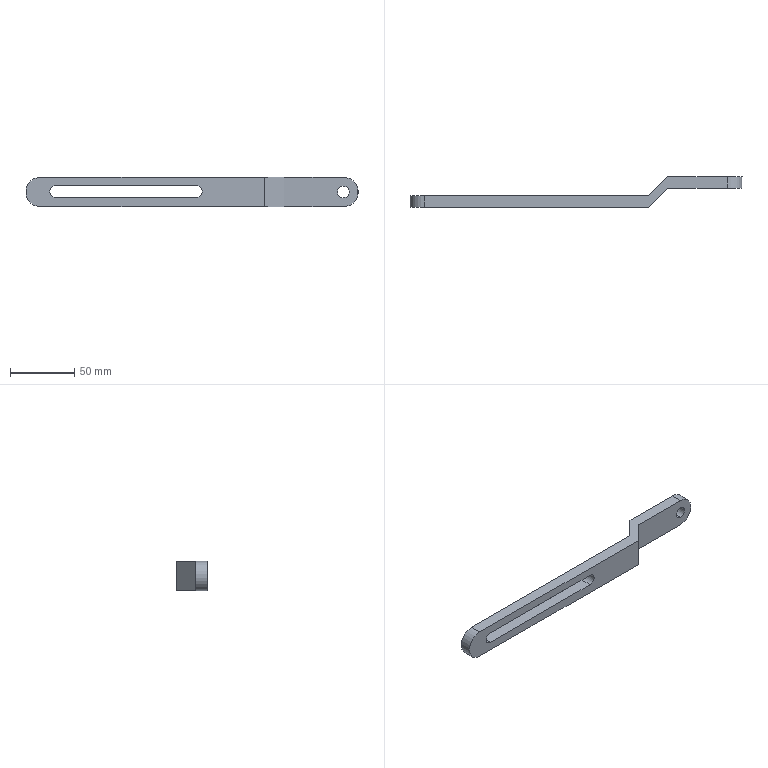Part | SolidWorks | features BaseBody 1 | 1 solid | 17 faces | box 258.849 x 23.849 x 23 mm | volume 42505 mm3 | plane 10 | cylinder 7 | commonest cylinder face diameters 9 x5 23 x2
STEP:
#1=CARTESIAN_POINT('',(247.349,14.849,7.));
#2=VERTEX_POINT('',#1);
#3=CARTESIAN_POINT('',(247.349,14.849,16.));
#4=VERTEX_POINT('',#3);
#5=CARTESIAN_POINT('',(247.349,14.849,11.5));
#6=DIRECTION('',(0.,-1.,0.));
#7=DIRECTION('',(0.,0.,-1.));
#8=AXIS2_PLACEMENT_3D('',#5,#6,#7);
#9=CIRCLE('',#8,4.5);
#10=EDGE_CURVE('',#2,#4,#9,.T.);
#11=ORIENTED_EDGE('',*,*,#10,.F.);
#12=CARTESIAN_POINT('',(247.349,5.849,7.));
#13=VERTEX_POINT('',#12);
#14=CARTESIAN_POINT('',(247.349,14.849,7.));
#15=DIRECTION('',(0.,-1.,0.));
#16=VECTOR('',#15,1000.);
#17=LINE('',#14,#16);
#18=EDGE_CURVE('',#2,#13,#17,.T.);
#19=ORIENTED_EDGE('',*,*,#18,.T.);
#20=CARTESIAN_POINT('',(247.349,5.849,16.));
#21=VERTEX_POINT('',#20);
#22=CARTESIAN_POINT('',(247.349,5.849,11.5));
#23=DIRECTION('',(0.,1.,0.));
#24=DIRECTION('',(-1.,0.,0.));
#25=AXIS2_PLACEMENT_3D('',#22,#23,#24);
#26=CIRCLE('',#25,4.5);
#27=EDGE_CURVE('',#21,#13,#26,.T.);
#28=ORIENTED_EDGE('',*,*,#27,.F.);
#29=CARTESIAN_POINT('',(247.349,14.849,16.));
#30=DIRECTION('',(0.,-1.,0.));
#31=VECTOR('',#30,1000.);
#32=LINE('',#29,#31);
#33=EDGE_CURVE('',#4,#21,#32,.T.);
#34=ORIENTED_EDGE('',*,*,#33,.F.);
#35=EDGE_LOOP('',(#11,#19,#28,#34));
#36=FACE_OUTER_BOUND('',#35,.T.);
#37=CARTESIAN_POINT('',(247.349,14.849,11.5));
#38=DIRECTION('',(0.,-1.,0.));
#39=DIRECTION('',(0.,0.,1.));
#40=AXIS2_PLACEMENT_3D('',#37,#38,#39);
#41=CYLINDRICAL_SURFACE('',#40,4.5);
#42=ADVANCED_FACE('',(#36),#41,.F.);
#43=CARTESIAN_POINT('',(22.998,-9.,16.35));
#44=VERTEX_POINT('',#43);
#45=CARTESIAN_POINT('',(23.,-9.,7.35));
#46=VERTEX_POINT('',#45);
#47=CARTESIAN_POINT('',(23.,-9.,11.85));
#48=DIRECTION('',(0.,-1.,0.));
#49=DIRECTION('',(-1.,0.,0.));
#50=AXIS2_PLACEMENT_3D('',#47,#48,#49);
#51=CIRCLE('',#50,4.5);
#52=EDGE_CURVE('',#44,#46,#51,.T.);
#53=ORIENTED_EDGE('',*,*,#52,.T.);
#54=CARTESIAN_POINT('',(23.,0.,7.35));
#55=VERTEX_POINT('',#54);
#56=CARTESIAN_POINT('',(23.,-23.,7.35));
#57=DIRECTION('',(0.,1.,0.));
#58=VECTOR('',#57,1000.);
#59=LINE('',#56,#58);
#60=EDGE_CURVE('',#46,#55,#59,.T.);
#61=ORIENTED_EDGE('',*,*,#60,.T.);
#62=CARTESIAN_POINT('',(22.998,0.,16.35));
#63=VERTEX_POINT('',#62);
#64=CARTESIAN_POINT('',(23.,0.,11.85));
#65=DIRECTION('',(0.,-1.,0.));
#66=DIRECTION('',(-1.,0.,0.));
#67=AXIS2_PLACEMENT_3D('',#64,#65,#66);
#68=CIRCLE('',#67,4.5);
#69=EDGE_CURVE('',#63,#55,#68,.T.);
#70=ORIENTED_EDGE('',*,*,#69,.F.);
#71=CARTESIAN_POINT('',(22.998,-23.,16.35));
#72=DIRECTION('',(0.,-1.,0.));
#73=VECTOR('',#72,1000.);
#74=LINE('',#71,#73);
#75=EDGE_CURVE('',#63,#44,#74,.T.);
#76=ORIENTED_EDGE('',*,*,#75,.T.);
#77=EDGE_LOOP('',(#53,#61,#70,#76));
#78=FACE_OUTER_BOUND('',#77,.T.);
#79=CARTESIAN_POINT('',(23.,-23.,11.85));
#80=DIRECTION('',(0.,1.,0.));
#81=DIRECTION('',(0.,0.,-1.));
#82=AXIS2_PLACEMENT_3D('',#79,#80,#81);
#83=CYLINDRICAL_SURFACE('',#82,4.5);
#84=ADVANCED_FACE('',(#78),#83,.F.);
#85=CARTESIAN_POINT('',(133.002,-9.,7.407));
#86=VERTEX_POINT('',#85);
#87=CARTESIAN_POINT('',(132.998,-9.,16.407));
#88=VERTEX_POINT('',#87);
#89=CARTESIAN_POINT('',(133.,-9.,11.907));
#90=DIRECTION('',(0.,-1.,0.));
#91=DIRECTION('',(-1.,0.,0.));
#92=AXIS2_PLACEMENT_3D('',#89,#90,#91);
#93=CIRCLE('',#92,4.5);
#94=EDGE_CURVE('',#86,#88,#93,.T.);
#95=ORIENTED_EDGE('',*,*,#94,.T.);
#96=CARTESIAN_POINT('',(132.998,0.,16.407));
#97=VERTEX_POINT('',#96);
#98=CARTESIAN_POINT('',(132.998,-23.,16.407));
#99=DIRECTION('',(0.,-1.,0.));
#100=VECTOR('',#99,1000.);
#101=LINE('',#98,#100);
#102=EDGE_CURVE('',#97,#88,#101,.T.);
#103=ORIENTED_EDGE('',*,*,#102,.F.);
#104=CARTESIAN_POINT('',(133.002,0.,7.407));
#105=VERTEX_POINT('',#104);
#106=CARTESIAN_POINT('',(133.,0.,11.907));
#107=DIRECTION('',(0.,-1.,0.));
#108=DIRECTION('',(-1.,0.,0.));
#109=AXIS2_PLACEMENT_3D('',#106,#107,#108);
#110=CIRCLE('',#109,4.5);
#111=EDGE_CURVE('',#105,#97,#110,.T.);
#112=ORIENTED_EDGE('',*,*,#111,.F.);
#113=CARTESIAN_POINT('',(133.002,-23.,7.407));
#114=DIRECTION('',(0.,-1.,0.));
#115=VECTOR('',#114,1000.);
#116=LINE('',#113,#115);
#117=EDGE_CURVE('',#105,#86,#116,.T.);
#118=ORIENTED_EDGE('',*,*,#117,.T.);
#119=EDGE_LOOP('',(#95,#103,#112,#118));
#120=FACE_OUTER_BOUND('',#119,.T.);
#121=CARTESIAN_POINT('',(133.,-23.,11.907));
#122=DIRECTION('',(0.,1.,0.));
#123=DIRECTION('',(0.,0.,-1.));
#124=AXIS2_PLACEMENT_3D('',#121,#122,#123);
#125=CYLINDRICAL_SURFACE('',#124,4.5);
#126=ADVANCED_FACE('',(#120),#125,.F.);
#127=CARTESIAN_POINT('',(23.002,-9.,7.35));
#128=VERTEX_POINT('',#127);
#129=CARTESIAN_POINT('',(0.008065,-9.,7.338));
#130=DIRECTION('',(1.,0.,0.000515));
#131=VECTOR('',#130,1000.);
#132=LINE('',#129,#131);
#133=EDGE_CURVE('',#128,#86,#132,.T.);
#134=ORIENTED_EDGE('',*,*,#133,.T.);
#135=ORIENTED_EDGE('',*,*,#117,.F.);
#136=CARTESIAN_POINT('',(23.002,0.,7.35));
#137=VERTEX_POINT('',#136);
#138=CARTESIAN_POINT('',(23.002,0.,7.35));
#139=DIRECTION('',(1.,0.,0.000515));
#140=VECTOR('',#139,1000.);
#141=LINE('',#138,#140);
#142=EDGE_CURVE('',#137,#105,#141,.T.);
#143=ORIENTED_EDGE('',*,*,#142,.F.);
#144=CARTESIAN_POINT('',(23.002,-23.,7.35));
#145=DIRECTION('',(0.,-1.,0.));
#146=VECTOR('',#145,1000.);
#147=LINE('',#144,#146);
#148=EDGE_CURVE('',#137,#128,#147,.T.);
#149=ORIENTED_EDGE('',*,*,#148,.T.);
#150=EDGE_LOOP('',(#134,#135,#143,#149));
#151=FACE_OUTER_BOUND('',#150,.T.);
#152=CARTESIAN_POINT('',(23.002,-23.,7.35));
#153=DIRECTION('',(-0.000515,0.,1.));
#154=DIRECTION('',(0.,1.,0.));
#155=AXIS2_PLACEMENT_3D('',#152,#153,#154);
#156=PLANE('',#155);
#157=ADVANCED_FACE('',(#151),#156,.T.);
#158=ORIENTED_EDGE('',*,*,#60,.F.);
#159=CARTESIAN_POINT('',(23.,-9.,11.85));
#160=DIRECTION('',(0.,-1.,0.));
#161=DIRECTION('',(-1.,0.,0.));
#162=AXIS2_PLACEMENT_3D('',#159,#160,#161);
#163=CIRCLE('',#162,4.5);
#164=EDGE_CURVE('',#46,#128,#163,.T.);
#165=ORIENTED_EDGE('',*,*,#164,.T.);
#166=ORIENTED_EDGE('',*,*,#148,.F.);
#167=CARTESIAN_POINT('',(23.,0.,11.85));
#168=DIRECTION('',(0.,-1.,0.));
#169=DIRECTION('',(-1.,0.,0.));
#170=AXIS2_PLACEMENT_3D('',#167,#168,#169);
#171=CIRCLE('',#170,4.5);
#172=EDGE_CURVE('',#55,#137,#171,.T.);
#173=ORIENTED_EDGE('',*,*,#172,.F.);
#174=EDGE_LOOP('',(#158,#165,#166,#173));
#175=FACE_OUTER_BOUND('',#174,.T.);
#176=CARTESIAN_POINT('',(23.,-23.,11.85));
#177=DIRECTION('',(0.,1.,0.));
#178=DIRECTION('',(0.,0.,-1.));
#179=AXIS2_PLACEMENT_3D('',#176,#177,#178);
#180=CYLINDRICAL_SURFACE('',#179,4.5);
#181=ADVANCED_FACE('',(#175),#180,.F.);
#182=CARTESIAN_POINT('',(0.003431,-9.,16.338));
#183=DIRECTION('',(-1.,0.,-0.000515));
#184=VECTOR('',#183,1000.);
#185=LINE('',#182,#184);
#186=EDGE_CURVE('',#88,#44,#185,.T.);
#187=ORIENTED_EDGE('',*,*,#186,.T.);
#188=ORIENTED_EDGE('',*,*,#75,.F.);
#189=CARTESIAN_POINT('',(132.998,0.,16.407));
#190=DIRECTION('',(-1.,0.,-0.000515));
#191=VECTOR('',#190,1000.);
#192=LINE('',#189,#191);
#193=EDGE_CURVE('',#97,#63,#192,.T.);
#194=ORIENTED_EDGE('',*,*,#193,.F.);
#195=ORIENTED_EDGE('',*,*,#102,.T.);
#196=EDGE_LOOP('',(#187,#188,#194,#195));
#197=FACE_OUTER_BOUND('',#196,.T.);
#198=CARTESIAN_POINT('',(132.998,-23.,16.407));
#199=DIRECTION('',(0.000515,0.,-1.));
#200=DIRECTION('',(0.,-1.,0.));
#201=AXIS2_PLACEMENT_3D('',#198,#199,#200);
#202=PLANE('',#201);
#203=ADVANCED_FACE('',(#197),#202,.T.);
#204=ORIENTED_EDGE('',*,*,#18,.F.);
#205=CARTESIAN_POINT('',(247.349,14.849,11.5));
#206=DIRECTION('',(0.,-1.,0.));
#207=DIRECTION('',(0.,0.,-1.));
#208=AXIS2_PLACEMENT_3D('',#205,#206,#207);
#209=CIRCLE('',#208,4.5);
#210=EDGE_CURVE('',#4,#2,#209,.T.);
#211=ORIENTED_EDGE('',*,*,#210,.F.);
#212=ORIENTED_EDGE('',*,*,#33,.T.);
#213=CARTESIAN_POINT('',(247.349,5.849,11.5));
#214=DIRECTION('',(0.,1.,0.));
#215=DIRECTION('',(-1.,0.,0.));
#216=AXIS2_PLACEMENT_3D('',#213,#214,#215);
#217=CIRCLE('',#216,4.5);
#218=EDGE_CURVE('',#13,#21,#217,.T.);
#219=ORIENTED_EDGE('',*,*,#218,.F.);
#220=EDGE_LOOP('',(#204,#211,#212,#219));
#221=FACE_OUTER_BOUND('',#220,.T.);
#222=CARTESIAN_POINT('',(247.349,14.849,11.5));
#223=DIRECTION('',(0.,-1.,0.));
#224=DIRECTION('',(0.,0.,1.));
#225=AXIS2_PLACEMENT_3D('',#222,#223,#224);
#226=CYLINDRICAL_SURFACE('',#225,4.5);
#227=ADVANCED_FACE('',(#221),#226,.F.);
#228=CARTESIAN_POINT('',(11.5,0.,0.));
#229=VERTEX_POINT('',#228);
#230=CARTESIAN_POINT('',(11.5,0.,23.));
#231=VERTEX_POINT('',#230);
#232=CARTESIAN_POINT('',(11.5,0.,11.5));
#233=DIRECTION('',(0.,1.,0.));
#234=DIRECTION('',(0.,0.,-1.));
#235=AXIS2_PLACEMENT_3D('',#232,#233,#234);
#236=CIRCLE('',#235,11.5);
#237=EDGE_CURVE('',#229,#231,#236,.T.);
#238=ORIENTED_EDGE('',*,*,#237,.F.);
#239=CARTESIAN_POINT('',(11.5,-9.,0.));
#240=VERTEX_POINT('',#239);
#241=CARTESIAN_POINT('',(11.5,0.,0.));
#242=DIRECTION('',(0.,1.,0.));
#243=VECTOR('',#242,1000.);
#244=LINE('',#241,#243);
#245=EDGE_CURVE('',#240,#229,#244,.T.);
#246=ORIENTED_EDGE('',*,*,#245,.F.);
#247=CARTESIAN_POINT('',(11.5,-9.,23.));
#248=VERTEX_POINT('',#247);
#249=CARTESIAN_POINT('',(11.5,-9.,11.5));
#250=DIRECTION('',(0.,-1.,0.));
#251=DIRECTION('',(-1.,0.,0.));
#252=AXIS2_PLACEMENT_3D('',#249,#250,#251);
#253=CIRCLE('',#252,11.5);
#254=EDGE_CURVE('',#248,#240,#253,.T.);
#255=ORIENTED_EDGE('',*,*,#254,.F.);
#256=CARTESIAN_POINT('',(11.5,-9.,23.));
#257=DIRECTION('',(0.,-1.,0.));
#258=VECTOR('',#257,1000.);
#259=LINE('',#256,#258);
#260=EDGE_CURVE('',#231,#248,#259,.T.);
#261=ORIENTED_EDGE('',*,*,#260,.F.);
#262=EDGE_LOOP('',(#238,#246,#255,#261));
#263=FACE_OUTER_BOUND('',#262,.T.);
#264=CARTESIAN_POINT('',(11.5,0.,11.5));
#265=DIRECTION('',(0.,1.,0.));
#266=DIRECTION('',(1.,0.,0.));
#267=AXIS2_PLACEMENT_3D('',#264,#265,#266);
#268=CYLINDRICAL_SURFACE('',#267,11.5);
#269=ADVANCED_FACE('',(#263),#268,.T.);
#270=CARTESIAN_POINT('',(247.349,5.849,0.));
#271=VERTEX_POINT('',#270);
#272=CARTESIAN_POINT('',(247.349,5.849,23.));
#273=VERTEX_POINT('',#272);
#274=CARTESIAN_POINT('',(247.349,5.849,11.5));
#275=DIRECTION('',(0.,-1.,0.));
#276=DIRECTION('',(-1.,0.,0.));
#277=AXIS2_PLACEMENT_3D('',#274,#275,#276);
#278=CIRCLE('',#277,11.5);
#279=EDGE_CURVE('',#271,#273,#278,.T.);
#280=ORIENTED_EDGE('',*,*,#279,.F.);
#281=CARTESIAN_POINT('',(247.349,14.849,0.));
#282=VERTEX_POINT('',#281);
#283=CARTESIAN_POINT('',(247.349,0.,0.));
#284=DIRECTION('',(0.,-1.,0.));
#285=VECTOR('',#284,1000.);
#286=LINE('',#283,#285);
#287=EDGE_CURVE('',#282,#271,#286,.T.);
#288=ORIENTED_EDGE('',*,*,#287,.F.);
#289=CARTESIAN_POINT('',(247.349,14.849,23.));
#290=VERTEX_POINT('',#289);
#291=CARTESIAN_POINT('',(247.349,14.849,11.5));
#292=DIRECTION('',(0.,1.,0.));
#293=DIRECTION('',(0.,0.,-1.));
#294=AXIS2_PLACEMENT_3D('',#291,#292,#293);
#295=CIRCLE('',#294,11.5);
#296=EDGE_CURVE('',#290,#282,#295,.T.);
#297=ORIENTED_EDGE('',*,*,#296,.F.);
#298=CARTESIAN_POINT('',(247.349,14.849,23.));
#299=DIRECTION('',(0.,1.,0.));
#300=VECTOR('',#299,1000.);
#301=LINE('',#298,#300);
#302=EDGE_CURVE('',#273,#290,#301,.T.);
#303=ORIENTED_EDGE('',*,*,#302,.F.);
#304=EDGE_LOOP('',(#280,#288,#297,#303));
#305=FACE_OUTER_BOUND('',#304,.T.);
#306=CARTESIAN_POINT('',(247.349,0.,11.5));
#307=DIRECTION('',(0.,-1.,0.));
#308=DIRECTION('',(-1.,0.,0.));
#309=AXIS2_PLACEMENT_3D('',#306,#307,#308);
#310=CYLINDRICAL_SURFACE('',#309,11.5);
#311=ADVANCED_FACE('',(#305),#310,.T.);
#312=CARTESIAN_POINT('',(186.,-9.,0.));
#313=VERTEX_POINT('',#312);
#314=CARTESIAN_POINT('',(0.,-9.,0.));
#315=DIRECTION('',(1.,0.,0.));
#316=VECTOR('',#315,1000.);
#317=LINE('',#314,#316);
#318=EDGE_CURVE('',#240,#313,#317,.T.);
#319=ORIENTED_EDGE('',*,*,#318,.F.);
#320=ORIENTED_EDGE('',*,*,#245,.T.);
#321=CARTESIAN_POINT('',(186.,0.,0.));
#322=VERTEX_POINT('',#321);
#323=CARTESIAN_POINT('',(186.,0.,0.));
#324=DIRECTION('',(-1.,0.,0.));
#325=VECTOR('',#324,1000.);
#326=LINE('',#323,#325);
#327=EDGE_CURVE('',#322,#229,#326,.T.);
#328=ORIENTED_EDGE('',*,*,#327,.F.);
#329=CARTESIAN_POINT('',(200.849,14.849,0.));
#330=VERTEX_POINT('',#329);
#331=CARTESIAN_POINT('',(200.849,14.849,0.));
#332=DIRECTION('',(-0.7071,-0.7071,0.));
#333=VECTOR('',#332,1000.);
#334=LINE('',#331,#333);
#335=EDGE_CURVE('',#330,#322,#334,.T.);
#336=ORIENTED_EDGE('',*,*,#335,.F.);
#337=CARTESIAN_POINT('',(258.849,14.849,0.));
#338=DIRECTION('',(-1.,0.,0.));
#339=VECTOR('',#338,1000.);
#340=LINE('',#337,#339);
#341=EDGE_CURVE('',#282,#330,#340,.T.);
#342=ORIENTED_EDGE('',*,*,#341,.F.);
#343=ORIENTED_EDGE('',*,*,#287,.T.);
#344=CARTESIAN_POINT('',(200.849,5.849,0.));
#345=VERTEX_POINT('',#344);
#346=CARTESIAN_POINT('',(200.849,5.849,0.));
#347=DIRECTION('',(1.,0.,0.));
#348=VECTOR('',#347,1000.);
#349=LINE('',#346,#348);
#350=EDGE_CURVE('',#345,#271,#349,.T.);
#351=ORIENTED_EDGE('',*,*,#350,.F.);
#352=CARTESIAN_POINT('',(186.,-9.,0.));
#353=DIRECTION('',(0.7071,0.7071,0.));
#354=VECTOR('',#353,1000.);
#355=LINE('',#352,#354);
#356=EDGE_CURVE('',#313,#345,#355,.T.);
#357=ORIENTED_EDGE('',*,*,#356,.F.);
#358=EDGE_LOOP('',(#319,#320,#328,#336,#342,#343,#351,#357));
#359=FACE_OUTER_BOUND('',#358,.T.);
#360=CARTESIAN_POINT('',(0.,0.,0.));
#361=DIRECTION('',(0.,0.,1.));
#362=DIRECTION('',(1.,0.,0.));
#363=AXIS2_PLACEMENT_3D('',#360,#361,#362);
#364=PLANE('',#363);
#365=ADVANCED_FACE('',(#359),#364,.F.);
#366=CARTESIAN_POINT('',(186.,0.,23.));
#367=VERTEX_POINT('',#366);
#368=CARTESIAN_POINT('',(186.,0.,23.));
#369=DIRECTION('',(-1.,0.,0.));
#370=VECTOR('',#369,1000.);
#371=LINE('',#368,#370);
#372=EDGE_CURVE('',#367,#231,#371,.T.);
#373=ORIENTED_EDGE('',*,*,#372,.T.);
#374=ORIENTED_EDGE('',*,*,#260,.T.);
#375=CARTESIAN_POINT('',(186.,-9.,23.));
#376=VERTEX_POINT('',#375);
#377=CARTESIAN_POINT('',(0.,-9.,23.));
#378=DIRECTION('',(1.,0.,0.));
#379=VECTOR('',#378,1000.);
#380=LINE('',#377,#379);
#381=EDGE_CURVE('',#248,#376,#380,.T.);
#382=ORIENTED_EDGE('',*,*,#381,.T.);
#383=CARTESIAN_POINT('',(200.849,5.849,23.));
#384=VERTEX_POINT('',#383);
#385=CARTESIAN_POINT('',(186.,-9.,23.));
#386=DIRECTION('',(0.7071,0.7071,0.));
#387=VECTOR('',#386,1000.);
#388=LINE('',#385,#387);
#389=EDGE_CURVE('',#376,#384,#388,.T.);
#390=ORIENTED_EDGE('',*,*,#389,.T.);
#391=CARTESIAN_POINT('',(200.849,5.849,23.));
#392=DIRECTION('',(1.,0.,0.));
#393=VECTOR('',#392,1000.);
#394=LINE('',#391,#393);
#395=EDGE_CURVE('',#384,#273,#394,.T.);
#396=ORIENTED_EDGE('',*,*,#395,.T.);
#397=ORIENTED_EDGE('',*,*,#302,.T.);
#398=CARTESIAN_POINT('',(200.849,14.849,23.));
#399=VERTEX_POINT('',#398);
#400=CARTESIAN_POINT('',(258.849,14.849,23.));
#401=DIRECTION('',(-1.,0.,0.));
#402=VECTOR('',#401,1000.);
#403=LINE('',#400,#402);
#404=EDGE_CURVE('',#290,#399,#403,.T.);
#405=ORIENTED_EDGE('',*,*,#404,.T.);
#406=CARTESIAN_POINT('',(200.849,14.849,23.));
#407=DIRECTION('',(-0.7071,-0.7071,0.));
#408=VECTOR('',#407,1000.);
#409=LINE('',#406,#408);
#410=EDGE_CURVE('',#399,#367,#409,.T.);
#411=ORIENTED_EDGE('',*,*,#410,.T.);
#412=EDGE_LOOP('',(#373,#374,#382,#390,#396,#397,#405,#411));
#413=FACE_OUTER_BOUND('',#412,.T.);
#414=CARTESIAN_POINT('',(0.,0.,23.));
#415=DIRECTION('',(0.,0.,1.));
#416=DIRECTION('',(1.,0.,0.));
#417=AXIS2_PLACEMENT_3D('',#414,#415,#416);
#418=PLANE('',#417);
#419=ADVANCED_FACE('',(#413),#418,.T.);
#420=ORIENTED_EDGE('',*,*,#335,.T.);
#421=CARTESIAN_POINT('',(186.,0.,23.));
#422=DIRECTION('',(0.,0.,-1.));
#423=VECTOR('',#422,1000.);
#424=LINE('',#421,#423);
#425=EDGE_CURVE('',#367,#322,#424,.T.);
#426=ORIENTED_EDGE('',*,*,#425,.F.);
#427=ORIENTED_EDGE('',*,*,#410,.F.);
#428=CARTESIAN_POINT('',(200.849,14.849,23.));
#429=DIRECTION('',(0.,0.,-1.));
#430=VECTOR('',#429,1000.);
#431=LINE('',#428,#430);
#432=EDGE_CURVE('',#399,#330,#431,.T.);
#433=ORIENTED_EDGE('',*,*,#432,.T.);
#434=EDGE_LOOP('',(#420,#426,#427,#433));
#435=FACE_OUTER_BOUND('',#434,.T.);
#436=CARTESIAN_POINT('',(200.849,14.849,23.));
#437=DIRECTION('',(0.7071,-0.7071,0.));
#438=DIRECTION('',(0.,0.,-1.));
#439=AXIS2_PLACEMENT_3D('',#436,#437,#438);
#440=PLANE('',#439);
#441=ADVANCED_FACE('',(#435),#440,.F.);
#442=ORIENTED_EDGE('',*,*,#296,.T.);
#443=ORIENTED_EDGE('',*,*,#341,.T.);
#444=ORIENTED_EDGE('',*,*,#432,.F.);
#445=ORIENTED_EDGE('',*,*,#404,.F.);
#446=EDGE_LOOP('',(#442,#443,#444,#445));
#447=FACE_OUTER_BOUND('',#446,.T.);
#448=ORIENTED_EDGE('',*,*,#210,.T.);
#449=ORIENTED_EDGE('',*,*,#10,.T.);
#450=EDGE_LOOP('',(#448,#449));
#451=FACE_BOUND('',#450,.T.);
#452=CARTESIAN_POINT('',(258.849,14.849,23.));
#453=DIRECTION('',(0.,-1.,0.));
#454=DIRECTION('',(0.,0.,-1.));
#455=AXIS2_PLACEMENT_3D('',#452,#453,#454);
#456=PLANE('',#455);
#457=ADVANCED_FACE('',(#447,#451),#456,.F.);
#458=ORIENTED_EDGE('',*,*,#350,.T.);
#459=ORIENTED_EDGE('',*,*,#279,.T.);
#460=ORIENTED_EDGE('',*,*,#395,.F.);
#461=CARTESIAN_POINT('',(200.849,5.849,23.));
#462=DIRECTION('',(0.,0.,-1.));
#463=VECTOR('',#462,1000.);
#464=LINE('',#461,#463);
#465=EDGE_CURVE('',#384,#345,#464,.T.);
#466=ORIENTED_EDGE('',*,*,#465,.T.);
#467=EDGE_LOOP('',(#458,#459,#460,#466));
#468=FACE_OUTER_BOUND('',#467,.T.);
#469=ORIENTED_EDGE('',*,*,#27,.T.);
#470=ORIENTED_EDGE('',*,*,#218,.T.);
#471=EDGE_LOOP('',(#469,#470));
#472=FACE_BOUND('',#471,.T.);
#473=CARTESIAN_POINT('',(200.849,5.849,23.));
#474=DIRECTION('',(0.,1.,0.));
#475=DIRECTION('',(1.,0.,0.));
#476=AXIS2_PLACEMENT_3D('',#473,#474,#475);
#477=PLANE('',#476);
#478=ADVANCED_FACE('',(#468,#472),#477,.F.);
#479=ORIENTED_EDGE('',*,*,#356,.T.);
#480=ORIENTED_EDGE('',*,*,#465,.F.);
#481=ORIENTED_EDGE('',*,*,#389,.F.);
#482=CARTESIAN_POINT('',(186.,-9.,23.));
#483=DIRECTION('',(0.,0.,-1.));
#484=VECTOR('',#483,1000.);
#485=LINE('',#482,#484);
#486=EDGE_CURVE('',#376,#313,#485,.T.);
#487=ORIENTED_EDGE('',*,*,#486,.T.);
#488=EDGE_LOOP('',(#479,#480,#481,#487));
#489=FACE_OUTER_BOUND('',#488,.T.);
#490=CARTESIAN_POINT('',(186.,-9.,23.));
#491=DIRECTION('',(-0.7071,0.7071,0.));
#492=DIRECTION('',(0.,0.,1.));
#493=AXIS2_PLACEMENT_3D('',#490,#491,#492);
#494=PLANE('',#493);
#495=ADVANCED_FACE('',(#489),#494,.F.);
#496=ORIENTED_EDGE('',*,*,#254,.T.);
#497=ORIENTED_EDGE('',*,*,#318,.T.);
#498=ORIENTED_EDGE('',*,*,#486,.F.);
#499=ORIENTED_EDGE('',*,*,#381,.F.);
#500=EDGE_LOOP('',(#496,#497,#498,#499));
#501=FACE_OUTER_BOUND('',#500,.T.);
#502=ORIENTED_EDGE('',*,*,#186,.F.);
#503=ORIENTED_EDGE('',*,*,#94,.F.);
#504=ORIENTED_EDGE('',*,*,#133,.F.);
#505=ORIENTED_EDGE('',*,*,#164,.F.);
#506=ORIENTED_EDGE('',*,*,#52,.F.);
#507=EDGE_LOOP('',(#502,#503,#504,#505,#506));
#508=FACE_BOUND('',#507,.T.);
#509=CARTESIAN_POINT('',(0.,-9.,23.));
#510=DIRECTION('',(0.,1.,0.));
#511=DIRECTION('',(1.,0.,0.));
#512=AXIS2_PLACEMENT_3D('',#509,#510,#511);
#513=PLANE('',#512);
#514=ADVANCED_FACE('',(#501,#508),#513,.F.);
#515=ORIENTED_EDGE('',*,*,#111,.T.);
#516=ORIENTED_EDGE('',*,*,#193,.T.);
#517=ORIENTED_EDGE('',*,*,#69,.T.);
#518=ORIENTED_EDGE('',*,*,#172,.T.);
#519=ORIENTED_EDGE('',*,*,#142,.T.);
#520=EDGE_LOOP('',(#515,#516,#517,#518,#519));
#521=FACE_BOUND('',#520,.T.);
#522=ORIENTED_EDGE('',*,*,#327,.T.);
#523=ORIENTED_EDGE('',*,*,#237,.T.);
#524=ORIENTED_EDGE('',*,*,#372,.F.);
#525=ORIENTED_EDGE('',*,*,#425,.T.);
#526=EDGE_LOOP('',(#522,#523,#524,#525));
#527=FACE_OUTER_BOUND('',#526,.T.);
#528=CARTESIAN_POINT('',(186.,0.,23.));
#529=DIRECTION('',(0.,-1.,0.));
#530=DIRECTION('',(0.,0.,-1.));
#531=AXIS2_PLACEMENT_3D('',#528,#529,#530);
#532=PLANE('',#531);
#533=ADVANCED_FACE('',(#521,#527),#532,.F.);
#534=CLOSED_SHELL('',(#42,#84,#126,#157,#181,#203,#227,#269,#311,#365,#419,#441,#457,#478,#495,#514,#533));
#535=MANIFOLD_SOLID_BREP('',#534);
#536=CARTESIAN_POINT('',(0.,0.,0.));
#537=DIRECTION('',(0.,0.,1.));
#538=DIRECTION('',(1.,0.,0.));
#539=AXIS2_PLACEMENT_3D('',#536,#537,#538);
#540=(LENGTH_UNIT()NAMED_UNIT(*)SI_UNIT(.MILLI.,.METRE.));
#541=UNCERTAINTY_MEASURE_WITH_UNIT(LENGTH_MEASURE(0.00001),#540,'','');
#542=(NAMED_UNIT(*)PLANE_ANGLE_UNIT()SI_UNIT($,.RADIAN.));
#543=(NAMED_UNIT(*)SI_UNIT($,.STERADIAN.)SOLID_ANGLE_UNIT());
#544=(GEOMETRIC_REPRESENTATION_CONTEXT(3)GLOBAL_UNCERTAINTY_ASSIGNED_CONTEXT((#541))GLOBAL_UNIT_ASSIGNED_CONTEXT((#540,#542,#543))REPRESENTATION_CONTEXT('',''));
#545=ADVANCED_BREP_SHAPE_REPRESENTATION('',(#535,#539),#544);